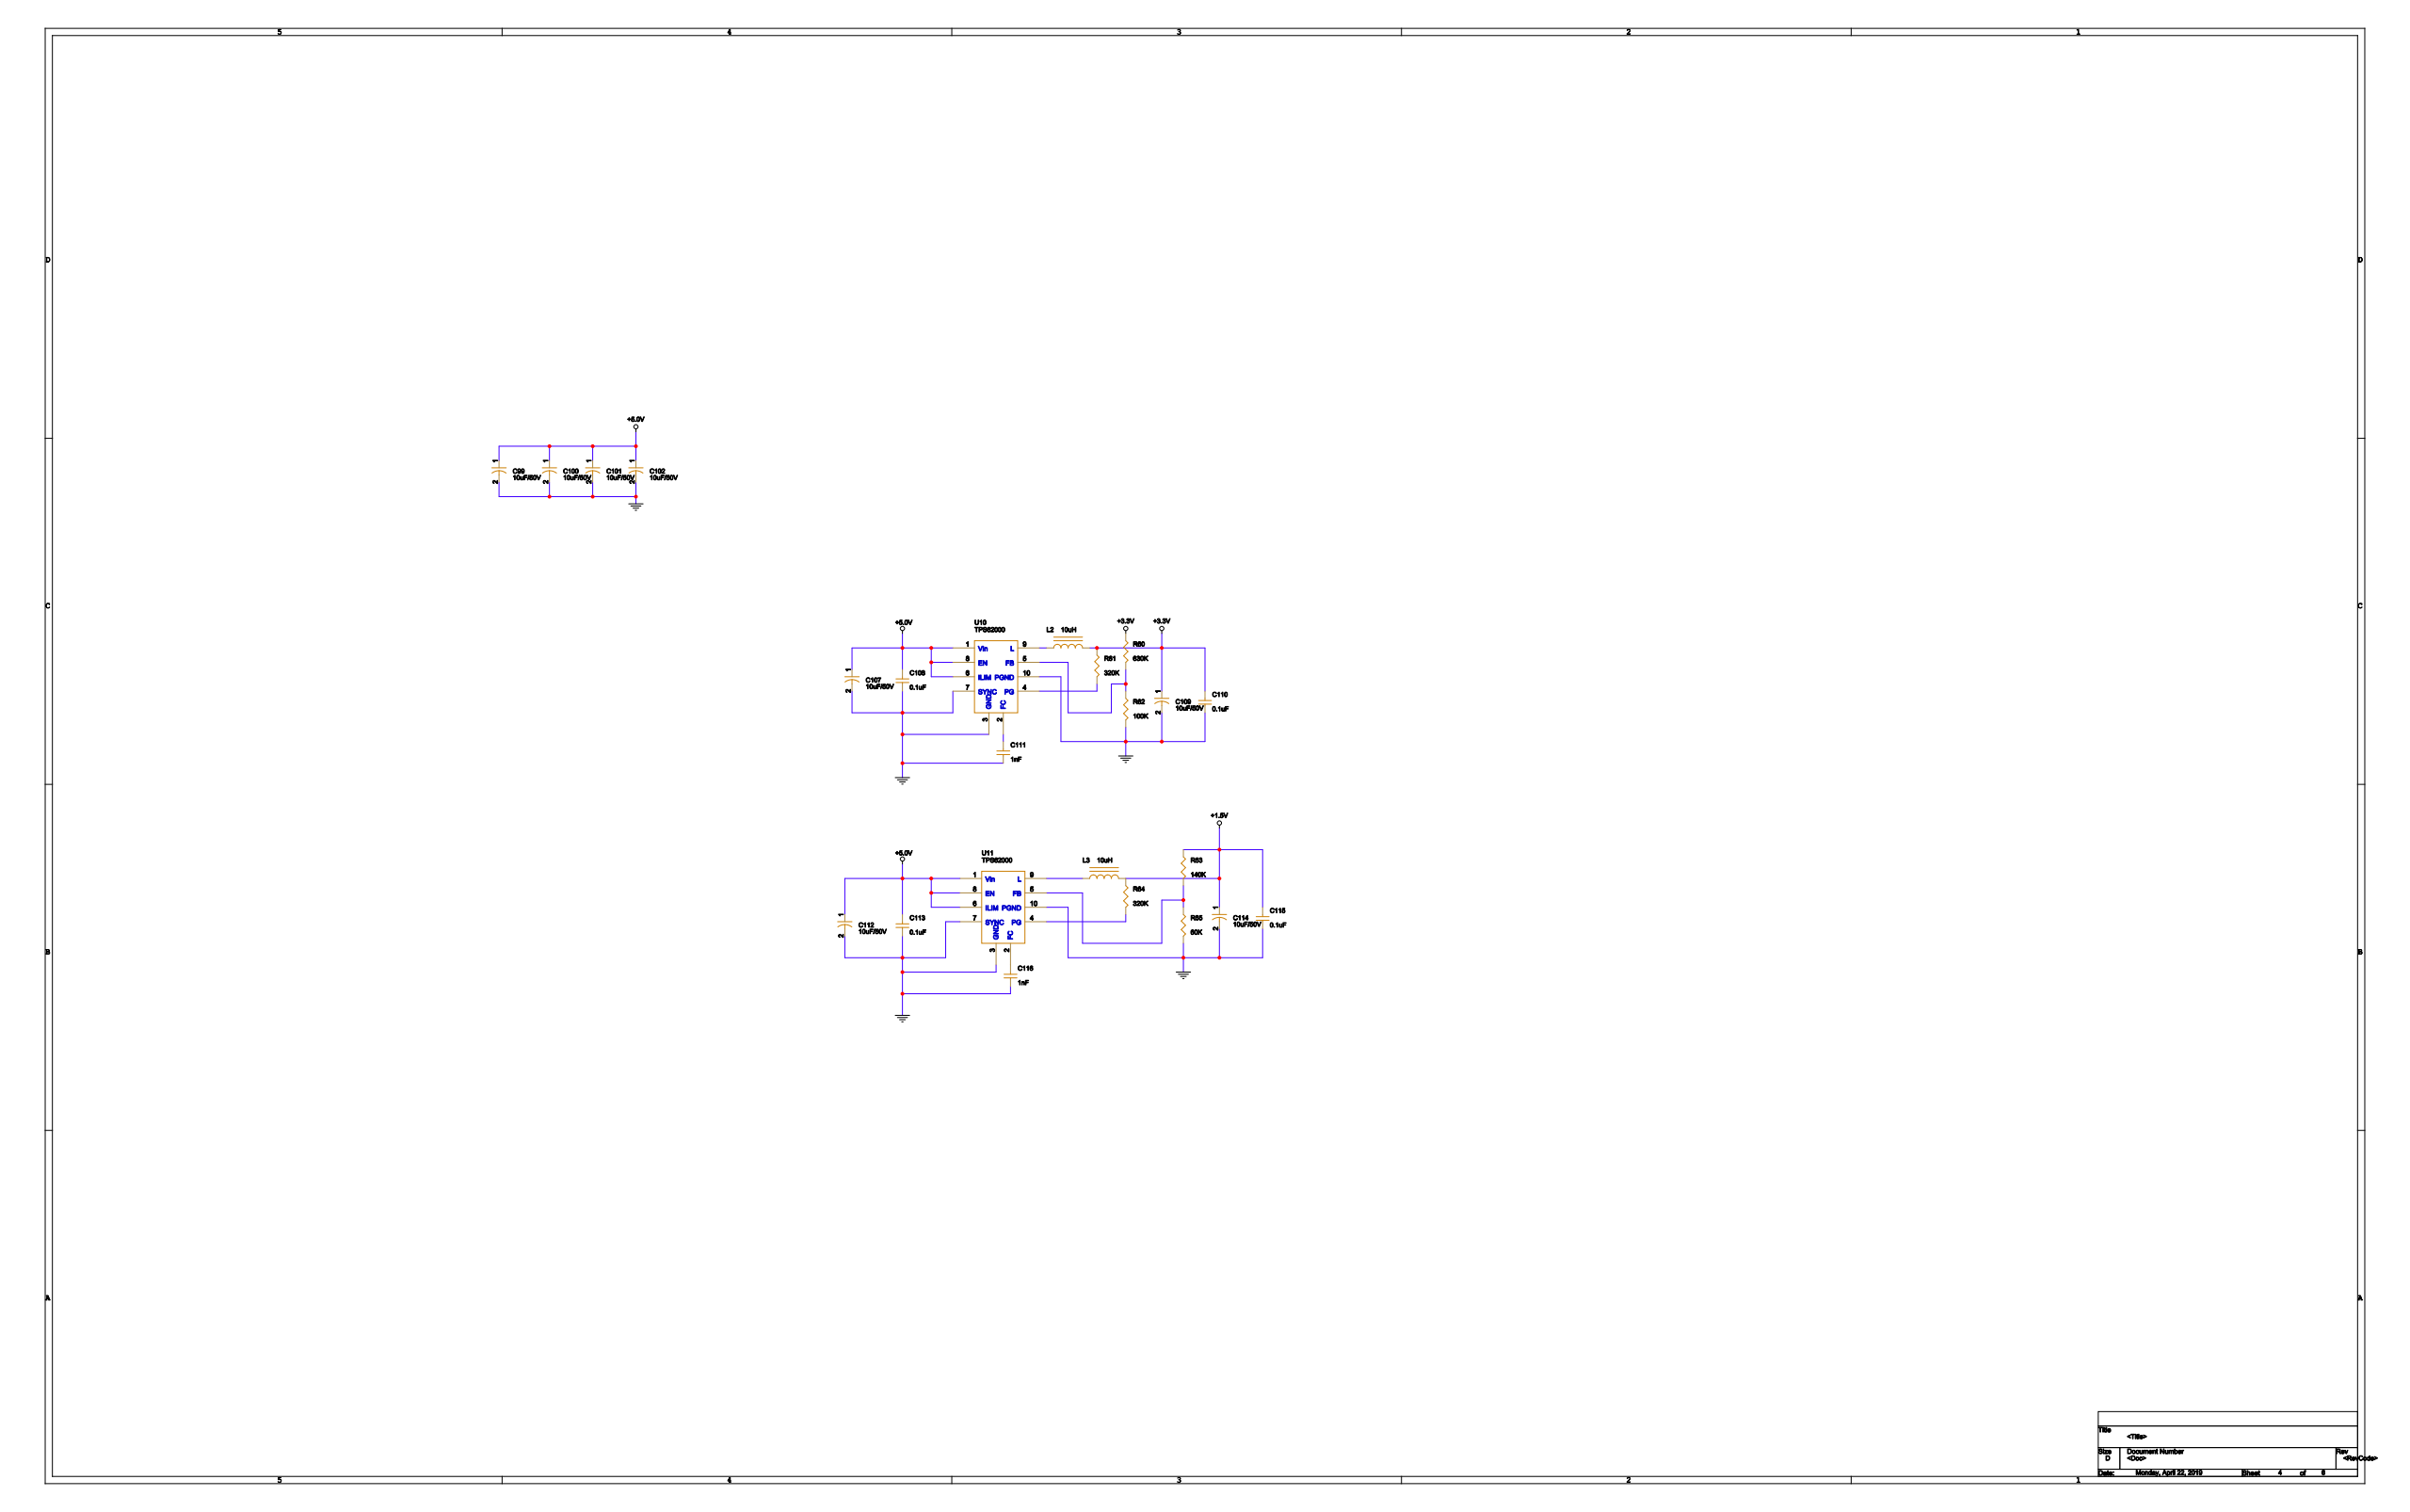Circuit board | Cadence Allegro | 362 parts | 391 nets | one sheet of the schematic
Parts on this sheet (reference | value | footprint):
C99 | 10uF/50V | 7343
C100 | 10uF/50V | 7343
C101 | 10uF/50V | 7343
C102 | 10uF/50V | 7343
C107 | 10uF/50V | 7343
C108 | 0.1uF | 1206
C109 | 10uF/50V | 7343
C110 | 0.1uF | 1206
C111 | 1nF | 1206
C112 | 10uF/50V | 7343
C113 | 0.1uF | 1206
C114 | 10uF/50V | 7343
C115 | 0.1uF | 1206
C116 | 1nF | 1206
L2 | 10uH | IND-SPD0735
L3 | 10uH | IND-SPD0735
R60 | 630K | 0805
R61 | 320K | 0805
R62 | 100K | 0805
R63 | 140K | 0805
R64 | 320K | 0805
R65 | 60K | 0805
U10 | TPS62000 | CFP10
U11 | TPS62000 | CFP10
Nets of these parts (net: part-pin ...):
+3.3V: C109-1 C110-2 L2-2 R60-1 R61-1
DGND: C99-2 C100-2 C101-2 C102-2 C107-2 C108-1 C109-2 C110-1 C111-1 C112-2 C113-1 C114-2 C115-1 C116-1 R62-2 R65-2 U10-3 U10-7 U10-10 U11-3 U11-7 U11-10
+5.0V: C99-1 C100-1 C101-1 C102-1 C107-1 C108-2 C112-1 C113-2 U10-1 U10-6 U10-8 U11-1 U11-6 U11-8
+1.5V: C114-1 C115-2 L3-2 R63-1 R64-1
N17253581: L3-1 U11-9
N17253585: L2-1 U10-9
N17253709: R63-2 R65-1 U11-5
N172536411: C116-2 U11-2
N17253785: R64-2 U11-4
N17253733: R60-2 R62-1 U10-5
N17253805: C111-2 U10-2
N17253623: R61-2 U10-4